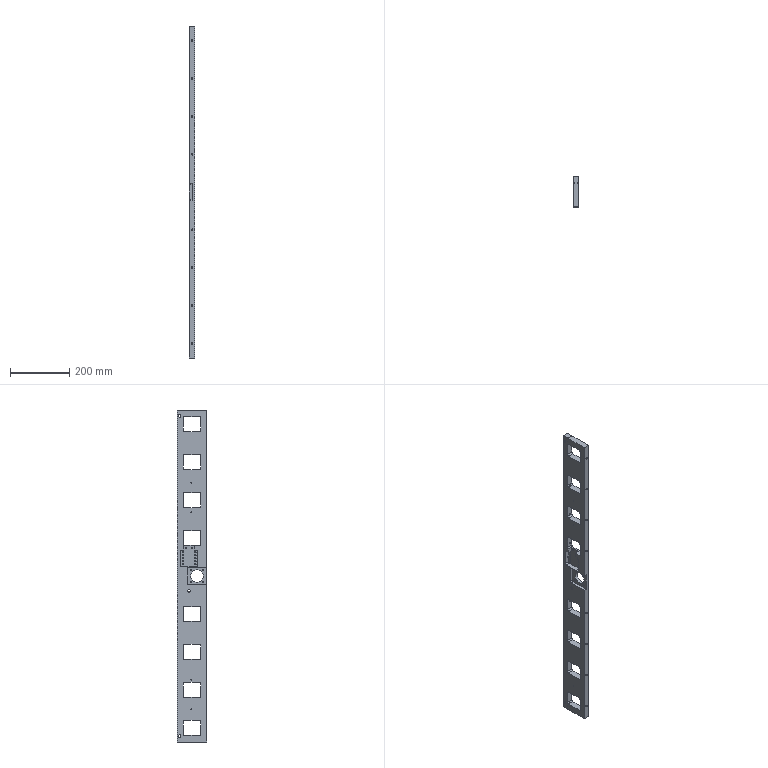Part | NX | 1 solid | 166 faces | box 20 x 100 x 1120 mm | volume 1637380 mm3 | cylinder 95 | plane 53 | cone 18 | commonest cylinder face diameters 10 x38 3.3 x25 4.2 x16 6.5 x8 5 x4 8.5 x3